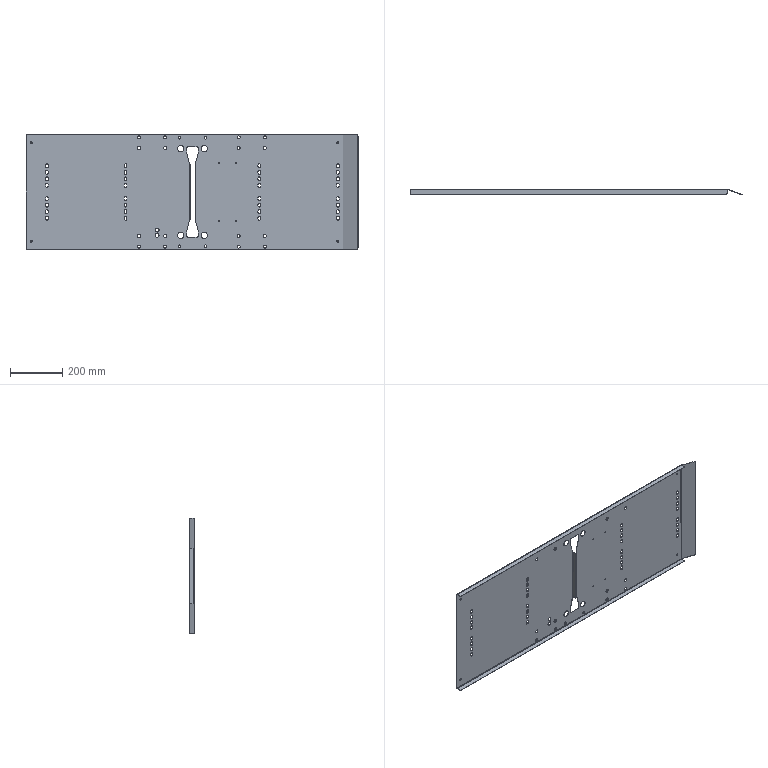Part | SolidWorks | features EdgeFlange 3, HoleWzd 3, LPattern 3, Fillet 2, ICE 2, FlatPattern 1, SMBaseFlange 1, SheetMetal 1 | 1 solid | 290 faces | box 1267 x 21.649 x 440.4 mm | volume 706056 mm3 | cylinder 182 | plane 108 | commonest cylinder face diameters 10 x114 12 x32 4.8 x8 7 x8 24 x8 15 x4